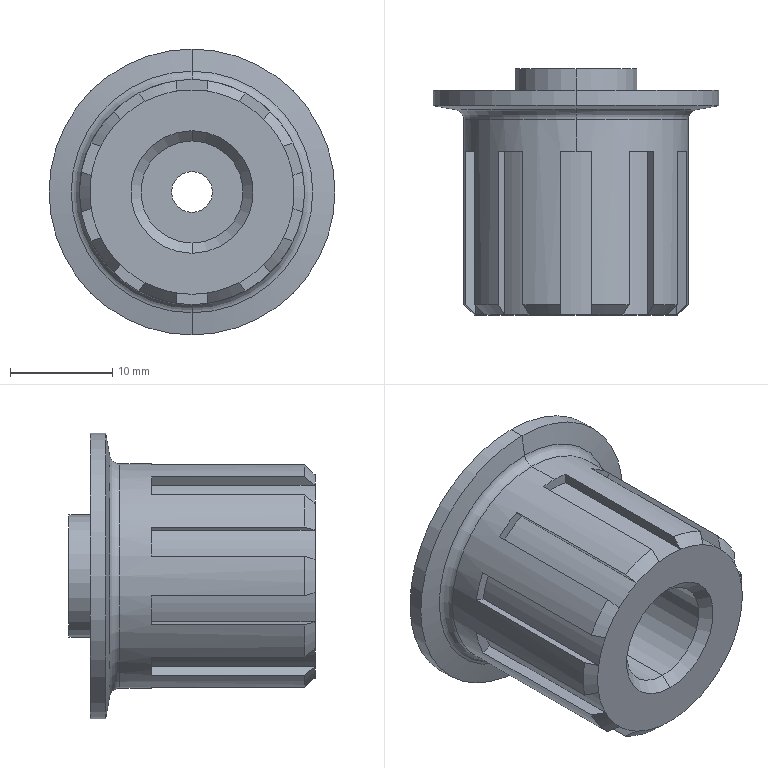Part | STEP file | AC40-04-KSTV-38JNR_AC3009A AL Drain-2 | 1 solid | 71 faces | box 28 x 24.1 x 28 mm | volume 7214 mm3 | plane 34 | cylinder 21 | cone 14 | torus 2 | commonest cylinder face diameters 20 x11 4 x2 10 x2 12 x2 22 x2 28 x2